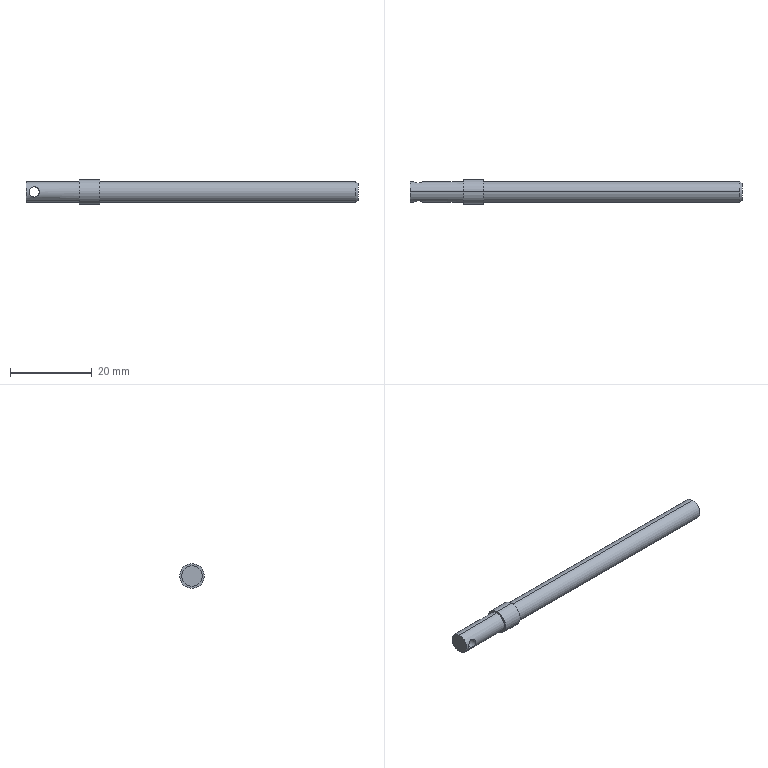Part | SolidWorks | features ICE 2, 3DProfileFeature 1, Chamfer 1, HoleWzd 1, Revolution 1 | 1 solid | 14 faces | box 81 x 6 x 6 mm | volume 1608 mm3 | cylinder 8 | plane 4 | cone 2 | commonest cylinder face diameters 5 x4 2.5 x2 6 x2
STEP:
#1=CARTESIAN_POINT('',(81.,0.,-2.));
#2=VERTEX_POINT('',#1);
#3=CARTESIAN_POINT('',(81.,0.,2.));
#4=VERTEX_POINT('',#3);
#5=CARTESIAN_POINT('',(81.,0.,0.));
#6=DIRECTION('',(1.,0.,0.));
#7=DIRECTION('',(0.,0.,-1.));
#8=AXIS2_PLACEMENT_3D('',#5,#6,#7);
#9=CIRCLE('',#8,2.);
#10=EDGE_CURVE('',#2,#4,#9,.T.);
#11=ORIENTED_EDGE('',*,*,#10,.F.);
#12=CARTESIAN_POINT('',(80.5,0.,-2.5));
#13=VERTEX_POINT('',#12);
#14=CARTESIAN_POINT('',(81.,0.,-2.));
#15=DIRECTION('',(-0.7071,0.,-0.7071));
#16=VECTOR('',#15,1000.);
#17=LINE('',#14,#16);
#18=EDGE_CURVE('',#2,#13,#17,.T.);
#19=ORIENTED_EDGE('',*,*,#18,.T.);
#20=CARTESIAN_POINT('',(80.5,0.,2.5));
#21=VERTEX_POINT('',#20);
#22=CARTESIAN_POINT('',(80.5,0.,0.));
#23=DIRECTION('',(-1.,0.,0.));
#24=DIRECTION('',(0.,0.,-1.));
#25=AXIS2_PLACEMENT_3D('',#22,#23,#24);
#26=CIRCLE('',#25,2.5);
#27=EDGE_CURVE('',#21,#13,#26,.T.);
#28=ORIENTED_EDGE('',*,*,#27,.F.);
#29=CARTESIAN_POINT('',(81.,0.,2.));
#30=DIRECTION('',(-0.7071,0.,0.7071));
#31=VECTOR('',#30,1000.);
#32=LINE('',#29,#31);
#33=EDGE_CURVE('',#4,#21,#32,.T.);
#34=ORIENTED_EDGE('',*,*,#33,.F.);
#35=EDGE_LOOP('',(#11,#19,#28,#34));
#36=FACE_OUTER_BOUND('',#35,.T.);
#37=CARTESIAN_POINT('',(81.,0.,0.));
#38=DIRECTION('',(-1.,0.,0.));
#39=DIRECTION('',(0.,0.,1.));
#40=AXIS2_PLACEMENT_3D('',#37,#38,#39);
#41=CONICAL_SURFACE('',#40,2.,0.7854);
#42=ADVANCED_FACE('',(#36),#41,.T.);
#43=CARTESIAN_POINT('',(2.,2.165,1.25));
#44=VERTEX_POINT('',#43);
#45=CARTESIAN_POINT('',(2.,2.165,-1.25));
#46=VERTEX_POINT('',#45);
#47=CARTESIAN_POINT('',(2.,2.165,1.25));
#48=CARTESIAN_POINT('',(1.917,2.165,1.25));
#49=CARTESIAN_POINT('',(1.833,2.17,1.242));
#50=CARTESIAN_POINT('',(1.671,2.188,1.209));
#51=CARTESIAN_POINT('',(1.593,2.202,1.185));
#52=CARTESIAN_POINT('',(1.365,2.251,1.089));
#53=CARTESIAN_POINT('',(1.23,2.296,0.9975));
#54=CARTESIAN_POINT('',(1.003,2.381,0.7704));
#55=CARTESIAN_POINT('',(0.9102,2.423,0.6335));
#56=CARTESIAN_POINT('',(0.7844,2.482,0.3335));
#57=CARTESIAN_POINT('',(0.7501,2.5,0.1666));
#58=CARTESIAN_POINT('',(0.7499,2.5,-0.1644));
#59=CARTESIAN_POINT('',(0.7835,2.483,-0.3311));
#60=CARTESIAN_POINT('',(0.9104,2.423,-0.6342));
#61=CARTESIAN_POINT('',(1.003,2.381,-0.7705));
#62=CARTESIAN_POINT('',(1.174,2.317,-0.9416));
#63=CARTESIAN_POINT('',(1.236,2.295,-0.9924));
#64=CARTESIAN_POINT('',(1.369,2.254,-1.082));
#65=CARTESIAN_POINT('',(1.442,2.235,-1.121));
#66=CARTESIAN_POINT('',(1.592,2.202,-1.184));
#67=CARTESIAN_POINT('',(1.67,2.189,-1.208));
#68=CARTESIAN_POINT('',(1.832,2.17,-1.241));
#69=CARTESIAN_POINT('',(1.916,2.165,-1.25));
#70=CARTESIAN_POINT('',(2.,2.165,-1.25));
#71=B_SPLINE_CURVE_WITH_KNOTS('',3,(#47,#48,#49,#50,#51,#52,#53,#54,#55,#56,#57,#58,#59,#60,#61,#62,#63,#64,#65,#66,#67,#68,#69,#70),.UNSPECIFIED.,.F.,.F.,(4,2,2,2,2,2,2,2,2,2,2,4),(0.003976,0.004224,0.004472,0.004968,0.005464,0.00596,0.006456,0.006952,0.0072,0.007448,0.007696,0.007944),.UNSPECIFIED.);
#72=EDGE_CURVE('',#44,#46,#71,.T.);
#73=ORIENTED_EDGE('',*,*,#72,.F.);
#74=CARTESIAN_POINT('',(2.,-2.165,1.25));
#75=VERTEX_POINT('',#74);
#76=CARTESIAN_POINT('',(2.,-2.5,1.25));
#77=DIRECTION('',(0.,-1.,0.));
#78=VECTOR('',#77,1000.);
#79=LINE('',#76,#78);
#80=EDGE_CURVE('',#44,#75,#79,.T.);
#81=ORIENTED_EDGE('',*,*,#80,.T.);
#82=CARTESIAN_POINT('',(2.,-2.165,-1.25));
#83=VERTEX_POINT('',#82);
#84=CARTESIAN_POINT('',(2.,-2.165,-1.25));
#85=CARTESIAN_POINT('',(1.916,-2.165,-1.25));
#86=CARTESIAN_POINT('',(1.833,-2.17,-1.242));
#87=CARTESIAN_POINT('',(1.672,-2.188,-1.209));
#88=CARTESIAN_POINT('',(1.592,-2.202,-1.184));
#89=CARTESIAN_POINT('',(1.366,-2.251,-1.09));
#90=CARTESIAN_POINT('',(1.23,-2.296,-0.9975));
#91=CARTESIAN_POINT('',(1.003,-2.381,-0.7709));
#92=CARTESIAN_POINT('',(0.9105,-2.423,-0.6341));
#93=CARTESIAN_POINT('',(0.8159,-2.468,-0.4087));
#94=CARTESIAN_POINT('',(0.7911,-2.48,-0.3285));
#95=CARTESIAN_POINT('',(0.7584,-2.496,-0.1663));
#96=CARTESIAN_POINT('',(0.7501,-2.5,-0.08412));
#97=CARTESIAN_POINT('',(0.7499,-2.5,0.1658));
#98=CARTESIAN_POINT('',(0.7838,-2.483,0.3322));
#99=CARTESIAN_POINT('',(0.9113,-2.423,0.6358));
#100=CARTESIAN_POINT('',(1.004,-2.381,0.7721));
#101=CARTESIAN_POINT('',(1.231,-2.295,0.9986));
#102=CARTESIAN_POINT('',(1.368,-2.251,1.091));
#103=CARTESIAN_POINT('',(1.667,-2.186,1.216));
#104=CARTESIAN_POINT('',(1.834,-2.165,1.25));
#105=CARTESIAN_POINT('',(2.,-2.165,1.25));
#106=B_SPLINE_CURVE_WITH_KNOTS('',3,(#84,#85,#86,#87,#88,#89,#90,#91,#92,#93,#94,#95,#96,#97,#98,#99,#100,#101,#102,#103,#104,#105),.UNSPECIFIED.,.F.,.F.,(4,2,2,2,2,2,2,2,2,2,4),(0.,0.0002485,0.000497,0.0009939,0.001491,0.001739,0.001988,0.002485,0.002982,0.003479,0.003976),.UNSPECIFIED.);
#107=EDGE_CURVE('',#83,#75,#106,.T.);
#108=ORIENTED_EDGE('',*,*,#107,.F.);
#109=CARTESIAN_POINT('',(2.,-2.5,-1.25));
#110=DIRECTION('',(0.,-1.,0.));
#111=VECTOR('',#110,1000.);
#112=LINE('',#109,#111);
#113=EDGE_CURVE('',#46,#83,#112,.T.);
#114=ORIENTED_EDGE('',*,*,#113,.F.);
#115=EDGE_LOOP('',(#73,#81,#108,#114));
#116=FACE_OUTER_BOUND('',#115,.T.);
#117=CARTESIAN_POINT('',(2.,-2.5,0.));
#118=DIRECTION('',(0.,-1.,0.));
#119=DIRECTION('',(0.,0.,-1.));
#120=AXIS2_PLACEMENT_3D('',#117,#118,#119);
#121=CYLINDRICAL_SURFACE('',#120,1.25);
#122=ADVANCED_FACE('',(#116),#121,.F.);
#123=ORIENTED_EDGE('',*,*,#27,.T.);
#124=CARTESIAN_POINT('',(18.,0.,-2.5));
#125=VERTEX_POINT('',#124);
#126=CARTESIAN_POINT('',(81.,0.,-2.5));
#127=DIRECTION('',(-1.,0.,0.));
#128=VECTOR('',#127,1000.);
#129=LINE('',#126,#128);
#130=EDGE_CURVE('',#13,#125,#129,.T.);
#131=ORIENTED_EDGE('',*,*,#130,.T.);
#132=CARTESIAN_POINT('',(18.,0.,2.5));
#133=VERTEX_POINT('',#132);
#134=CARTESIAN_POINT('',(18.,0.,0.));
#135=DIRECTION('',(1.,0.,0.));
#136=DIRECTION('',(0.,0.,-1.));
#137=AXIS2_PLACEMENT_3D('',#134,#135,#136);
#138=CIRCLE('',#137,2.5);
#139=EDGE_CURVE('',#125,#133,#138,.T.);
#140=ORIENTED_EDGE('',*,*,#139,.T.);
#141=CARTESIAN_POINT('',(81.,0.,2.5));
#142=DIRECTION('',(-1.,0.,0.));
#143=VECTOR('',#142,1000.);
#144=LINE('',#141,#143);
#145=EDGE_CURVE('',#21,#133,#144,.T.);
#146=ORIENTED_EDGE('',*,*,#145,.F.);
#147=EDGE_LOOP('',(#123,#131,#140,#146));
#148=FACE_OUTER_BOUND('',#147,.T.);
#149=CARTESIAN_POINT('',(81.,0.,0.));
#150=DIRECTION('',(-1.,0.,0.));
#151=DIRECTION('',(0.,0.,1.));
#152=AXIS2_PLACEMENT_3D('',#149,#150,#151);
#153=CYLINDRICAL_SURFACE('',#152,2.5);
#154=ADVANCED_FACE('',(#148),#153,.T.);
#155=CARTESIAN_POINT('',(2.,2.165,-1.25));
#156=CARTESIAN_POINT('',(2.084,2.165,-1.25));
#157=CARTESIAN_POINT('',(2.167,2.17,-1.242));
#158=CARTESIAN_POINT('',(2.328,2.188,-1.209));
#159=CARTESIAN_POINT('',(2.408,2.202,-1.184));
#160=CARTESIAN_POINT('',(2.634,2.251,-1.09));
#161=CARTESIAN_POINT('',(2.77,2.296,-0.9975));
#162=CARTESIAN_POINT('',(2.997,2.381,-0.7709));
#163=CARTESIAN_POINT('',(3.09,2.423,-0.6341));
#164=CARTESIAN_POINT('',(3.184,2.468,-0.4087));
#165=CARTESIAN_POINT('',(3.209,2.48,-0.3285));
#166=CARTESIAN_POINT('',(3.242,2.496,-0.1663));
#167=CARTESIAN_POINT('',(3.25,2.5,-0.08412));
#168=CARTESIAN_POINT('',(3.25,2.5,0.1658));
#169=CARTESIAN_POINT('',(3.216,2.483,0.3322));
#170=CARTESIAN_POINT('',(3.089,2.423,0.6358));
#171=CARTESIAN_POINT('',(2.996,2.381,0.7721));
#172=CARTESIAN_POINT('',(2.769,2.295,0.9986));
#173=CARTESIAN_POINT('',(2.632,2.251,1.091));
#174=CARTESIAN_POINT('',(2.333,2.186,1.216));
#175=CARTESIAN_POINT('',(2.166,2.165,1.25));
#176=CARTESIAN_POINT('',(2.,2.165,1.25));
#177=B_SPLINE_CURVE_WITH_KNOTS('',3,(#155,#156,#157,#158,#159,#160,#161,#162,#163,#164,#165,#166,#167,#168,#169,#170,#171,#172,#173,#174,#175,#176),.UNSPECIFIED.,.F.,.F.,(4,2,2,2,2,2,2,2,2,2,4),(0.,0.0002485,0.000497,0.0009939,0.001491,0.001739,0.001988,0.002485,0.002982,0.003479,0.003976),.UNSPECIFIED.);
#178=EDGE_CURVE('',#46,#44,#177,.T.);
#179=ORIENTED_EDGE('',*,*,#178,.T.);
#180=ORIENTED_EDGE('',*,*,#72,.T.);
#181=EDGE_LOOP('',(#179,#180));
#182=FACE_BOUND('',#181,.T.);
#183=CARTESIAN_POINT('',(0.,0.,2.5));
#184=VERTEX_POINT('',#183);
#185=CARTESIAN_POINT('',(0.,0.,-2.5));
#186=VERTEX_POINT('',#185);
#187=CARTESIAN_POINT('',(0.,0.,0.));
#188=DIRECTION('',(-1.,0.,0.));
#189=DIRECTION('',(0.,0.,1.));
#190=AXIS2_PLACEMENT_3D('',#187,#188,#189);
#191=CIRCLE('',#190,2.5);
#192=EDGE_CURVE('',#184,#186,#191,.T.);
#193=ORIENTED_EDGE('',*,*,#192,.F.);
#194=CARTESIAN_POINT('',(13.,0.,2.5));
#195=VERTEX_POINT('',#194);
#196=CARTESIAN_POINT('',(0.,0.,2.5));
#197=DIRECTION('',(1.,0.,0.));
#198=VECTOR('',#197,1000.);
#199=LINE('',#196,#198);
#200=EDGE_CURVE('',#184,#195,#199,.T.);
#201=ORIENTED_EDGE('',*,*,#200,.T.);
#202=CARTESIAN_POINT('',(13.,0.,-2.5));
#203=VERTEX_POINT('',#202);
#204=CARTESIAN_POINT('',(13.,0.,0.));
#205=DIRECTION('',(-1.,0.,0.));
#206=DIRECTION('',(0.,0.,1.));
#207=AXIS2_PLACEMENT_3D('',#204,#205,#206);
#208=CIRCLE('',#207,2.5);
#209=EDGE_CURVE('',#195,#203,#208,.T.);
#210=ORIENTED_EDGE('',*,*,#209,.T.);
#211=CARTESIAN_POINT('',(0.,0.,-2.5));
#212=DIRECTION('',(1.,0.,0.));
#213=VECTOR('',#212,1000.);
#214=LINE('',#211,#213);
#215=EDGE_CURVE('',#186,#203,#214,.T.);
#216=ORIENTED_EDGE('',*,*,#215,.F.);
#217=EDGE_LOOP('',(#193,#201,#210,#216));
#218=FACE_OUTER_BOUND('',#217,.T.);
#219=CARTESIAN_POINT('',(0.,0.,0.));
#220=DIRECTION('',(1.,0.,0.));
#221=DIRECTION('',(0.,0.,-1.));
#222=AXIS2_PLACEMENT_3D('',#219,#220,#221);
#223=CYLINDRICAL_SURFACE('',#222,2.5);
#224=ADVANCED_FACE('',(#182,#218),#223,.T.);
#225=CARTESIAN_POINT('',(18.,0.,3.));
#226=VERTEX_POINT('',#225);
#227=CARTESIAN_POINT('',(18.,0.,-3.));
#228=VERTEX_POINT('',#227);
#229=CARTESIAN_POINT('',(18.,0.,0.));
#230=DIRECTION('',(-1.,0.,0.));
#231=DIRECTION('',(0.,0.,1.));
#232=AXIS2_PLACEMENT_3D('',#229,#230,#231);
#233=CIRCLE('',#232,3.);
#234=EDGE_CURVE('',#226,#228,#233,.T.);
#235=ORIENTED_EDGE('',*,*,#234,.T.);
#236=CARTESIAN_POINT('',(13.,0.,-3.));
#237=VERTEX_POINT('',#236);
#238=CARTESIAN_POINT('',(18.,0.,-3.));
#239=DIRECTION('',(-1.,0.,0.));
#240=VECTOR('',#239,1000.);
#241=LINE('',#238,#240);
#242=EDGE_CURVE('',#228,#237,#241,.T.);
#243=ORIENTED_EDGE('',*,*,#242,.T.);
#244=CARTESIAN_POINT('',(13.,0.,3.));
#245=VERTEX_POINT('',#244);
#246=CARTESIAN_POINT('',(13.,0.,0.));
#247=DIRECTION('',(-1.,0.,0.));
#248=DIRECTION('',(0.,0.,1.));
#249=AXIS2_PLACEMENT_3D('',#246,#247,#248);
#250=CIRCLE('',#249,3.);
#251=EDGE_CURVE('',#245,#237,#250,.T.);
#252=ORIENTED_EDGE('',*,*,#251,.F.);
#253=CARTESIAN_POINT('',(18.,0.,3.));
#254=DIRECTION('',(-1.,0.,0.));
#255=VECTOR('',#254,1000.);
#256=LINE('',#253,#255);
#257=EDGE_CURVE('',#226,#245,#256,.T.);
#258=ORIENTED_EDGE('',*,*,#257,.F.);
#259=EDGE_LOOP('',(#235,#243,#252,#258));
#260=FACE_OUTER_BOUND('',#259,.T.);
#261=CARTESIAN_POINT('',(18.,0.,0.));
#262=DIRECTION('',(-1.,0.,0.));
#263=DIRECTION('',(0.,0.,1.));
#264=AXIS2_PLACEMENT_3D('',#261,#262,#263);
#265=CYLINDRICAL_SURFACE('',#264,3.);
#266=ADVANCED_FACE('',(#260),#265,.T.);
#267=ORIENTED_EDGE('',*,*,#242,.F.);
#268=CARTESIAN_POINT('',(18.,0.,0.));
#269=DIRECTION('',(-1.,0.,0.));
#270=DIRECTION('',(0.,0.,1.));
#271=AXIS2_PLACEMENT_3D('',#268,#269,#270);
#272=CIRCLE('',#271,3.);
#273=EDGE_CURVE('',#228,#226,#272,.T.);
#274=ORIENTED_EDGE('',*,*,#273,.T.);
#275=ORIENTED_EDGE('',*,*,#257,.T.);
#276=CARTESIAN_POINT('',(13.,0.,0.));
#277=DIRECTION('',(-1.,0.,0.));
#278=DIRECTION('',(0.,0.,1.));
#279=AXIS2_PLACEMENT_3D('',#276,#277,#278);
#280=CIRCLE('',#279,3.);
#281=EDGE_CURVE('',#237,#245,#280,.T.);
#282=ORIENTED_EDGE('',*,*,#281,.F.);
#283=EDGE_LOOP('',(#267,#274,#275,#282));
#284=FACE_OUTER_BOUND('',#283,.T.);
#285=CARTESIAN_POINT('',(18.,0.,0.));
#286=DIRECTION('',(-1.,0.,0.));
#287=DIRECTION('',(0.,0.,1.));
#288=AXIS2_PLACEMENT_3D('',#285,#286,#287);
#289=CYLINDRICAL_SURFACE('',#288,3.);
#290=ADVANCED_FACE('',(#284),#289,.T.);
#291=CARTESIAN_POINT('',(18.,0.,0.));
#292=DIRECTION('',(1.,0.,0.));
#293=DIRECTION('',(0.,0.,-1.));
#294=AXIS2_PLACEMENT_3D('',#291,#292,#293);
#295=CIRCLE('',#294,2.5);
#296=EDGE_CURVE('',#133,#125,#295,.T.);
#297=ORIENTED_EDGE('',*,*,#296,.F.);
#298=ORIENTED_EDGE('',*,*,#139,.F.);
#299=EDGE_LOOP('',(#297,#298));
#300=FACE_BOUND('',#299,.T.);
#301=ORIENTED_EDGE('',*,*,#234,.F.);
#302=ORIENTED_EDGE('',*,*,#273,.F.);
#303=EDGE_LOOP('',(#301,#302));
#304=FACE_OUTER_BOUND('',#303,.T.);
#305=CARTESIAN_POINT('',(18.,3.,0.));
#306=DIRECTION('',(1.,0.,0.));
#307=DIRECTION('',(0.,0.,-1.));
#308=AXIS2_PLACEMENT_3D('',#305,#306,#307);
#309=PLANE('',#308);
#310=ADVANCED_FACE('',(#300,#304),#309,.T.);
#311=CARTESIAN_POINT('',(13.,0.,0.));
#312=DIRECTION('',(-1.,0.,0.));
#313=DIRECTION('',(0.,0.,1.));
#314=AXIS2_PLACEMENT_3D('',#311,#312,#313);
#315=CIRCLE('',#314,2.5);
#316=EDGE_CURVE('',#203,#195,#315,.T.);
#317=ORIENTED_EDGE('',*,*,#316,.F.);
#318=ORIENTED_EDGE('',*,*,#209,.F.);
#319=EDGE_LOOP('',(#317,#318));
#320=FACE_BOUND('',#319,.T.);
#321=ORIENTED_EDGE('',*,*,#251,.T.);
#322=ORIENTED_EDGE('',*,*,#281,.T.);
#323=EDGE_LOOP('',(#321,#322));
#324=FACE_OUTER_BOUND('',#323,.T.);
#325=CARTESIAN_POINT('',(13.,0.,0.));
#326=DIRECTION('',(-1.,0.,0.));
#327=DIRECTION('',(0.,0.,1.));
#328=AXIS2_PLACEMENT_3D('',#325,#326,#327);
#329=PLANE('',#328);
#330=ADVANCED_FACE('',(#320,#324),#329,.T.);
#331=ORIENTED_EDGE('',*,*,#200,.F.);
#332=CARTESIAN_POINT('',(0.,0.,0.));
#333=DIRECTION('',(-1.,0.,0.));
#334=DIRECTION('',(0.,0.,1.));
#335=AXIS2_PLACEMENT_3D('',#332,#333,#334);
#336=CIRCLE('',#335,2.5);
#337=EDGE_CURVE('',#186,#184,#336,.T.);
#338=ORIENTED_EDGE('',*,*,#337,.F.);
#339=ORIENTED_EDGE('',*,*,#215,.T.);
#340=ORIENTED_EDGE('',*,*,#316,.T.);
#341=EDGE_LOOP('',(#331,#338,#339,#340));
#342=FACE_OUTER_BOUND('',#341,.T.);
#343=ORIENTED_EDGE('',*,*,#107,.T.);
#344=CARTESIAN_POINT('',(2.,-2.165,1.25));
#345=CARTESIAN_POINT('',(2.083,-2.165,1.25));
#346=CARTESIAN_POINT('',(2.167,-2.17,1.242));
#347=CARTESIAN_POINT('',(2.329,-2.188,1.209));
#348=CARTESIAN_POINT('',(2.407,-2.202,1.185));
#349=CARTESIAN_POINT('',(2.635,-2.251,1.089));
#350=CARTESIAN_POINT('',(2.77,-2.296,0.9975));
#351=CARTESIAN_POINT('',(2.997,-2.381,0.7704));
#352=CARTESIAN_POINT('',(3.09,-2.423,0.6335));
#353=CARTESIAN_POINT('',(3.216,-2.482,0.3335));
#354=CARTESIAN_POINT('',(3.25,-2.5,0.1666));
#355=CARTESIAN_POINT('',(3.25,-2.5,-0.1644));
#356=CARTESIAN_POINT('',(3.216,-2.483,-0.3311));
#357=CARTESIAN_POINT('',(3.09,-2.423,-0.6342));
#358=CARTESIAN_POINT('',(2.997,-2.381,-0.7705));
#359=CARTESIAN_POINT('',(2.826,-2.317,-0.9416));
#360=CARTESIAN_POINT('',(2.764,-2.295,-0.9924));
#361=CARTESIAN_POINT('',(2.631,-2.254,-1.082));
#362=CARTESIAN_POINT('',(2.558,-2.235,-1.121));
#363=CARTESIAN_POINT('',(2.408,-2.202,-1.184));
#364=CARTESIAN_POINT('',(2.33,-2.189,-1.208));
#365=CARTESIAN_POINT('',(2.168,-2.17,-1.241));
#366=CARTESIAN_POINT('',(2.084,-2.165,-1.25));
#367=CARTESIAN_POINT('',(2.,-2.165,-1.25));
#368=B_SPLINE_CURVE_WITH_KNOTS('',3,(#344,#345,#346,#347,#348,#349,#350,#351,#352,#353,#354,#355,#356,#357,#358,#359,#360,#361,#362,#363,#364,#365,#366,#367),.UNSPECIFIED.,.F.,.F.,(4,2,2,2,2,2,2,2,2,2,2,4),(0.003976,0.004224,0.004472,0.004968,0.005464,0.00596,0.006456,0.006952,0.0072,0.007448,0.007696,0.007944),.UNSPECIFIED.);
#369=EDGE_CURVE('',#75,#83,#368,.T.);
#370=ORIENTED_EDGE('',*,*,#369,.T.);
#371=EDGE_LOOP('',(#343,#370));
#372=FACE_BOUND('',#371,.T.);
#373=CARTESIAN_POINT('',(0.,0.,0.));
#374=DIRECTION('',(1.,0.,0.));
#375=DIRECTION('',(0.,0.,-1.));
#376=AXIS2_PLACEMENT_3D('',#373,#374,#375);
#377=CYLINDRICAL_SURFACE('',#376,2.5);
#378=ADVANCED_FACE('',(#342,#372),#377,.T.);
#379=ORIENTED_EDGE('',*,*,#337,.T.);
#380=ORIENTED_EDGE('',*,*,#192,.T.);
#381=EDGE_LOOP('',(#379,#380));
#382=FACE_OUTER_BOUND('',#381,.T.);
#383=CARTESIAN_POINT('',(0.,0.,0.));
#384=DIRECTION('',(-1.,0.,0.));
#385=DIRECTION('',(0.,0.,1.));
#386=AXIS2_PLACEMENT_3D('',#383,#384,#385);
#387=PLANE('',#386);
#388=ADVANCED_FACE('',(#382),#387,.T.);
#389=ORIENTED_EDGE('',*,*,#130,.F.);
#390=CARTESIAN_POINT('',(80.5,0.,0.));
#391=DIRECTION('',(-1.,0.,0.));
#392=DIRECTION('',(0.,0.,-1.));
#393=AXIS2_PLACEMENT_3D('',#390,#391,#392);
#394=CIRCLE('',#393,2.5);
#395=EDGE_CURVE('',#13,#21,#394,.T.);
#396=ORIENTED_EDGE('',*,*,#395,.T.);
#397=ORIENTED_EDGE('',*,*,#145,.T.);
#398=ORIENTED_EDGE('',*,*,#296,.T.);
#399=EDGE_LOOP('',(#389,#396,#397,#398));
#400=FACE_OUTER_BOUND('',#399,.T.);
#401=CARTESIAN_POINT('',(81.,0.,0.));
#402=DIRECTION('',(-1.,0.,0.));
#403=DIRECTION('',(0.,0.,1.));
#404=AXIS2_PLACEMENT_3D('',#401,#402,#403);
#405=CYLINDRICAL_SURFACE('',#404,2.5);
#406=ADVANCED_FACE('',(#400),#405,.T.);
#407=CARTESIAN_POINT('',(81.,0.,0.));
#408=DIRECTION('',(1.,0.,0.));
#409=DIRECTION('',(0.,0.,-1.));
#410=AXIS2_PLACEMENT_3D('',#407,#408,#409);
#411=CIRCLE('',#410,2.);
#412=EDGE_CURVE('',#4,#2,#411,.T.);
#413=ORIENTED_EDGE('',*,*,#412,.T.);
#414=ORIENTED_EDGE('',*,*,#10,.T.);
#415=EDGE_LOOP('',(#413,#414));
#416=FACE_OUTER_BOUND('',#415,.T.);
#417=CARTESIAN_POINT('',(81.,0.,0.));
#418=DIRECTION('',(1.,0.,0.));
#419=DIRECTION('',(0.,0.,-1.));
#420=AXIS2_PLACEMENT_3D('',#417,#418,#419);
#421=PLANE('',#420);
#422=ADVANCED_FACE('',(#416),#421,.T.);
#423=ORIENTED_EDGE('',*,*,#80,.F.);
#424=ORIENTED_EDGE('',*,*,#178,.F.);
#425=ORIENTED_EDGE('',*,*,#113,.T.);
#426=ORIENTED_EDGE('',*,*,#369,.F.);
#427=EDGE_LOOP('',(#423,#424,#425,#426));
#428=FACE_OUTER_BOUND('',#427,.T.);
#429=CARTESIAN_POINT('',(2.,-2.5,0.));
#430=DIRECTION('',(0.,-1.,0.));
#431=DIRECTION('',(0.,0.,-1.));
#432=AXIS2_PLACEMENT_3D('',#429,#430,#431);
#433=CYLINDRICAL_SURFACE('',#432,1.25);
#434=ADVANCED_FACE('',(#428),#433,.F.);
#435=ORIENTED_EDGE('',*,*,#18,.F.);
#436=ORIENTED_EDGE('',*,*,#412,.F.);
#437=ORIENTED_EDGE('',*,*,#33,.T.);
#438=ORIENTED_EDGE('',*,*,#395,.F.);
#439=EDGE_LOOP('',(#435,#436,#437,#438));
#440=FACE_OUTER_BOUND('',#439,.T.);
#441=CARTESIAN_POINT('',(81.,0.,0.));
#442=DIRECTION('',(-1.,0.,0.));
#443=DIRECTION('',(0.,0.,1.));
#444=AXIS2_PLACEMENT_3D('',#441,#442,#443);
#445=CONICAL_SURFACE('',#444,2.,0.7854);
#446=ADVANCED_FACE('',(#440),#445,.T.);
#447=CLOSED_SHELL('',(#42,#122,#154,#224,#266,#290,#310,#330,#378,#388,#406,#422,#434,#446));
#448=MANIFOLD_SOLID_BREP('',#447);
#449=CARTESIAN_POINT('',(0.,0.,0.));
#450=DIRECTION('',(0.,0.,1.));
#451=DIRECTION('',(1.,0.,0.));
#452=AXIS2_PLACEMENT_3D('',#449,#450,#451);
#453=(LENGTH_UNIT()NAMED_UNIT(*)SI_UNIT(.MILLI.,.METRE.));
#454=UNCERTAINTY_MEASURE_WITH_UNIT(LENGTH_MEASURE(0.00001),#453,'','');
#455=(NAMED_UNIT(*)PLANE_ANGLE_UNIT()SI_UNIT($,.RADIAN.));
#456=(NAMED_UNIT(*)SI_UNIT($,.STERADIAN.)SOLID_ANGLE_UNIT());
#457=(GEOMETRIC_REPRESENTATION_CONTEXT(3)GLOBAL_UNCERTAINTY_ASSIGNED_CONTEXT((#454))GLOBAL_UNIT_ASSIGNED_CONTEXT((#453,#455,#456))REPRESENTATION_CONTEXT('',''));
#458=ADVANCED_BREP_SHAPE_REPRESENTATION('',(#448,#452),#457);